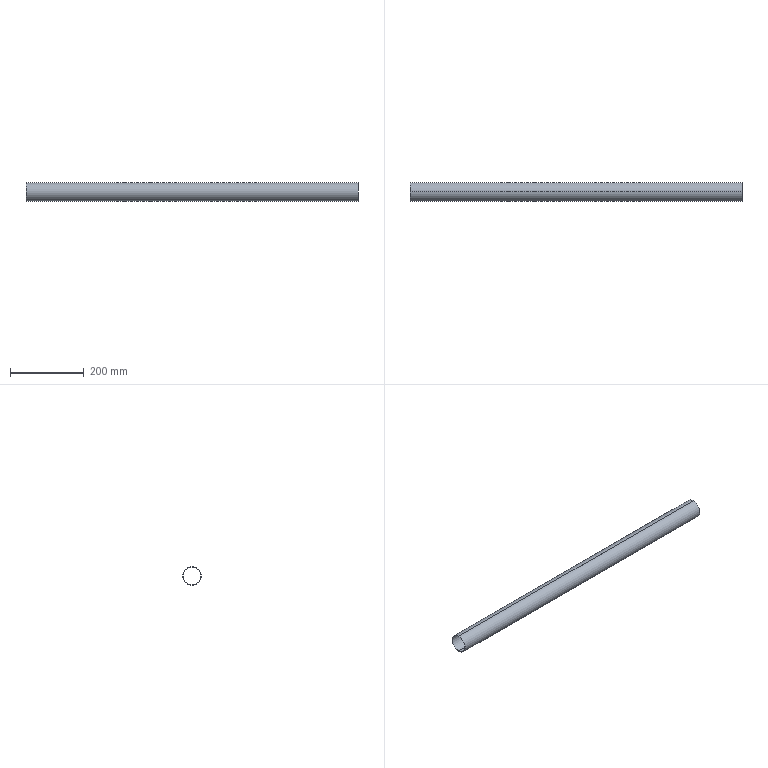Part | SolidWorks | features BaseBody 1 | 1 solid | 6 faces | box 898.8 x 50 x 50 mm | volume 165354 mm3 | cylinder 4 | plane 2 | commonest cylinder face diameters 47.6 x2 50 x2
STEP:
#1=CARTESIAN_POINT('',(898.8,0.,-23.8));
#2=VERTEX_POINT('',#1);
#3=CARTESIAN_POINT('',(898.8,0.,23.8));
#4=VERTEX_POINT('',#3);
#5=CARTESIAN_POINT('',(898.8,0.,0.));
#6=DIRECTION('',(-1.,0.,0.));
#7=DIRECTION('',(0.,0.,1.));
#8=AXIS2_PLACEMENT_3D('',#5,#6,#7);
#9=CIRCLE('',#8,23.8);
#10=EDGE_CURVE('',#2,#4,#9,.T.);
#11=ORIENTED_EDGE('',*,*,#10,.F.);
#12=CARTESIAN_POINT('',(0.,0.,-23.8));
#13=VERTEX_POINT('',#12);
#14=CARTESIAN_POINT('',(-133.939,0.,-23.8));
#15=DIRECTION('',(-1.,0.,0.));
#16=VECTOR('',#15,1000.);
#17=LINE('',#14,#16);
#18=EDGE_CURVE('',#2,#13,#17,.T.);
#19=ORIENTED_EDGE('',*,*,#18,.T.);
#20=CARTESIAN_POINT('',(0.,0.,23.8));
#21=VERTEX_POINT('',#20);
#22=CARTESIAN_POINT('',(0.,0.,0.));
#23=DIRECTION('',(-1.,0.,0.));
#24=DIRECTION('',(0.,0.,-1.));
#25=AXIS2_PLACEMENT_3D('',#22,#23,#24);
#26=CIRCLE('',#25,23.8);
#27=EDGE_CURVE('',#13,#21,#26,.T.);
#28=ORIENTED_EDGE('',*,*,#27,.T.);
#29=CARTESIAN_POINT('',(-133.939,0.,23.8));
#30=DIRECTION('',(-1.,0.,0.));
#31=VECTOR('',#30,1000.);
#32=LINE('',#29,#31);
#33=EDGE_CURVE('',#4,#21,#32,.T.);
#34=ORIENTED_EDGE('',*,*,#33,.F.);
#35=EDGE_LOOP('',(#11,#19,#28,#34));
#36=FACE_OUTER_BOUND('',#35,.T.);
#37=CARTESIAN_POINT('',(-133.939,0.,0.));
#38=DIRECTION('',(-1.,0.,0.));
#39=DIRECTION('',(0.,0.,1.));
#40=AXIS2_PLACEMENT_3D('',#37,#38,#39);
#41=CYLINDRICAL_SURFACE('',#40,23.8);
#42=ADVANCED_FACE('',(#36),#41,.F.);
#43=CARTESIAN_POINT('',(898.8,0.,25.));
#44=VERTEX_POINT('',#43);
#45=CARTESIAN_POINT('',(898.8,0.,-25.));
#46=VERTEX_POINT('',#45);
#47=CARTESIAN_POINT('',(898.8,0.,0.));
#48=DIRECTION('',(-1.,0.,0.));
#49=DIRECTION('',(0.,0.,1.));
#50=AXIS2_PLACEMENT_3D('',#47,#48,#49);
#51=CIRCLE('',#50,25.);
#52=EDGE_CURVE('',#44,#46,#51,.T.);
#53=ORIENTED_EDGE('',*,*,#52,.T.);
#54=CARTESIAN_POINT('',(0.,0.,-25.));
#55=VERTEX_POINT('',#54);
#56=CARTESIAN_POINT('',(-133.939,0.,-25.));
#57=DIRECTION('',(-1.,0.,0.));
#58=VECTOR('',#57,1000.);
#59=LINE('',#56,#58);
#60=EDGE_CURVE('',#46,#55,#59,.T.);
#61=ORIENTED_EDGE('',*,*,#60,.T.);
#62=CARTESIAN_POINT('',(0.,0.,25.));
#63=VERTEX_POINT('',#62);
#64=CARTESIAN_POINT('',(0.,0.,0.));
#65=DIRECTION('',(-1.,0.,0.));
#66=DIRECTION('',(0.,0.,1.));
#67=AXIS2_PLACEMENT_3D('',#64,#65,#66);
#68=CIRCLE('',#67,25.);
#69=EDGE_CURVE('',#63,#55,#68,.T.);
#70=ORIENTED_EDGE('',*,*,#69,.F.);
#71=CARTESIAN_POINT('',(-133.939,0.,25.));
#72=DIRECTION('',(-1.,0.,0.));
#73=VECTOR('',#72,1000.);
#74=LINE('',#71,#73);
#75=EDGE_CURVE('',#44,#63,#74,.T.);
#76=ORIENTED_EDGE('',*,*,#75,.F.);
#77=EDGE_LOOP('',(#53,#61,#70,#76));
#78=FACE_OUTER_BOUND('',#77,.T.);
#79=CARTESIAN_POINT('',(-133.939,0.,0.));
#80=DIRECTION('',(-1.,0.,0.));
#81=DIRECTION('',(0.,0.,1.));
#82=AXIS2_PLACEMENT_3D('',#79,#80,#81);
#83=CYLINDRICAL_SURFACE('',#82,25.);
#84=ADVANCED_FACE('',(#78),#83,.T.);
#85=CARTESIAN_POINT('',(0.,0.,0.));
#86=DIRECTION('',(-1.,0.,0.));
#87=DIRECTION('',(0.,0.,-1.));
#88=AXIS2_PLACEMENT_3D('',#85,#86,#87);
#89=CIRCLE('',#88,23.8);
#90=EDGE_CURVE('',#21,#13,#89,.T.);
#91=ORIENTED_EDGE('',*,*,#90,.F.);
#92=ORIENTED_EDGE('',*,*,#27,.F.);
#93=EDGE_LOOP('',(#91,#92));
#94=FACE_BOUND('',#93,.T.);
#95=ORIENTED_EDGE('',*,*,#69,.T.);
#96=CARTESIAN_POINT('',(0.,0.,0.));
#97=DIRECTION('',(-1.,0.,0.));
#98=DIRECTION('',(0.,0.,1.));
#99=AXIS2_PLACEMENT_3D('',#96,#97,#98);
#100=CIRCLE('',#99,25.);
#101=EDGE_CURVE('',#55,#63,#100,.T.);
#102=ORIENTED_EDGE('',*,*,#101,.T.);
#103=EDGE_LOOP('',(#95,#102));
#104=FACE_OUTER_BOUND('',#103,.T.);
#105=CARTESIAN_POINT('',(0.,0.,0.));
#106=DIRECTION('',(1.,0.,0.));
#107=DIRECTION('',(0.,0.,-1.));
#108=AXIS2_PLACEMENT_3D('',#105,#106,#107);
#109=PLANE('',#108);
#110=ADVANCED_FACE('',(#94,#104),#109,.F.);
#111=ORIENTED_EDGE('',*,*,#60,.F.);
#112=CARTESIAN_POINT('',(898.8,0.,0.));
#113=DIRECTION('',(-1.,0.,0.));
#114=DIRECTION('',(0.,0.,1.));
#115=AXIS2_PLACEMENT_3D('',#112,#113,#114);
#116=CIRCLE('',#115,25.);
#117=EDGE_CURVE('',#46,#44,#116,.T.);
#118=ORIENTED_EDGE('',*,*,#117,.T.);
#119=ORIENTED_EDGE('',*,*,#75,.T.);
#120=ORIENTED_EDGE('',*,*,#101,.F.);
#121=EDGE_LOOP('',(#111,#118,#119,#120));
#122=FACE_OUTER_BOUND('',#121,.T.);
#123=CARTESIAN_POINT('',(-133.939,0.,0.));
#124=DIRECTION('',(-1.,0.,0.));
#125=DIRECTION('',(0.,0.,1.));
#126=AXIS2_PLACEMENT_3D('',#123,#124,#125);
#127=CYLINDRICAL_SURFACE('',#126,25.);
#128=ADVANCED_FACE('',(#122),#127,.T.);
#129=CARTESIAN_POINT('',(898.8,0.,0.));
#130=DIRECTION('',(-1.,0.,0.));
#131=DIRECTION('',(0.,0.,1.));
#132=AXIS2_PLACEMENT_3D('',#129,#130,#131);
#133=CIRCLE('',#132,23.8);
#134=EDGE_CURVE('',#4,#2,#133,.T.);
#135=ORIENTED_EDGE('',*,*,#134,.T.);
#136=ORIENTED_EDGE('',*,*,#10,.T.);
#137=EDGE_LOOP('',(#135,#136));
#138=FACE_BOUND('',#137,.T.);
#139=ORIENTED_EDGE('',*,*,#52,.F.);
#140=ORIENTED_EDGE('',*,*,#117,.F.);
#141=EDGE_LOOP('',(#139,#140));
#142=FACE_OUTER_BOUND('',#141,.T.);
#143=CARTESIAN_POINT('',(898.8,25.,0.));
#144=DIRECTION('',(-1.,0.,0.));
#145=DIRECTION('',(0.,0.,1.));
#146=AXIS2_PLACEMENT_3D('',#143,#144,#145);
#147=PLANE('',#146);
#148=ADVANCED_FACE('',(#138,#142),#147,.F.);
#149=ORIENTED_EDGE('',*,*,#18,.F.);
#150=ORIENTED_EDGE('',*,*,#134,.F.);
#151=ORIENTED_EDGE('',*,*,#33,.T.);
#152=ORIENTED_EDGE('',*,*,#90,.T.);
#153=EDGE_LOOP('',(#149,#150,#151,#152));
#154=FACE_OUTER_BOUND('',#153,.T.);
#155=CARTESIAN_POINT('',(-133.939,0.,0.));
#156=DIRECTION('',(-1.,0.,0.));
#157=DIRECTION('',(0.,0.,1.));
#158=AXIS2_PLACEMENT_3D('',#155,#156,#157);
#159=CYLINDRICAL_SURFACE('',#158,23.8);
#160=ADVANCED_FACE('',(#154),#159,.F.);
#161=CLOSED_SHELL('',(#42,#84,#110,#128,#148,#160));
#162=MANIFOLD_SOLID_BREP('',#161);
#163=CARTESIAN_POINT('',(0.,0.,0.));
#164=DIRECTION('',(0.,0.,1.));
#165=DIRECTION('',(1.,0.,0.));
#166=AXIS2_PLACEMENT_3D('',#163,#164,#165);
#167=(LENGTH_UNIT()NAMED_UNIT(*)SI_UNIT(.MILLI.,.METRE.));
#168=UNCERTAINTY_MEASURE_WITH_UNIT(LENGTH_MEASURE(0.00001),#167,'','');
#169=(NAMED_UNIT(*)PLANE_ANGLE_UNIT()SI_UNIT($,.RADIAN.));
#170=(NAMED_UNIT(*)SI_UNIT($,.STERADIAN.)SOLID_ANGLE_UNIT());
#171=(GEOMETRIC_REPRESENTATION_CONTEXT(3)GLOBAL_UNCERTAINTY_ASSIGNED_CONTEXT((#168))GLOBAL_UNIT_ASSIGNED_CONTEXT((#167,#169,#170))REPRESENTATION_CONTEXT('',''));
#172=ADVANCED_BREP_SHAPE_REPRESENTATION('',(#162,#166),#171);